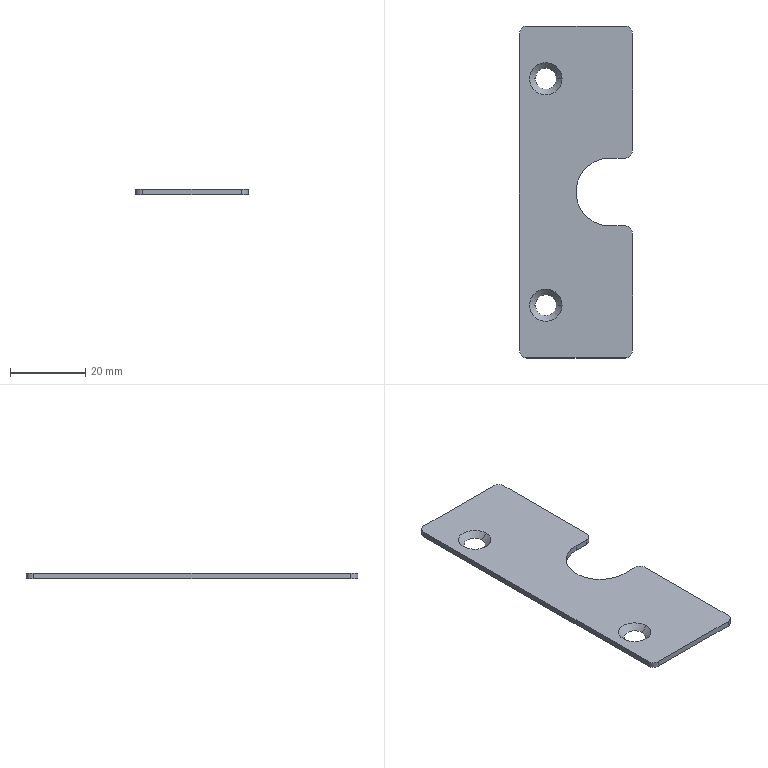Part | SolidWorks | features Chamfer 1, Fillet 1, FlatPattern 1, ICE 1, SMBaseFlange 1, SheetMetal 1 | 1 solid | 20 faces | box 30 x 88 x 1.5 mm | volume 3479 mm3 | plane 9 | cylinder 7 | cone 4 | commonest cylinder face diameters 4 x6 18 x1
STEP:
#1=CARTESIAN_POINT('',(-10.8,30.,-1.5));
#2=VERTEX_POINT('',#1);
#3=CARTESIAN_POINT('',(-5.2,30.,-1.5));
#4=VERTEX_POINT('',#3);
#5=CARTESIAN_POINT('',(-8.,30.,-1.5));
#6=DIRECTION('',(0.,0.,1.));
#7=DIRECTION('',(1.,0.,0.));
#8=AXIS2_PLACEMENT_3D('',#5,#6,#7);
#9=CIRCLE('',#8,2.8);
#10=EDGE_CURVE('',#2,#4,#9,.T.);
#11=ORIENTED_EDGE('',*,*,#10,.F.);
#12=CARTESIAN_POINT('',(-12.3,30.,0.));
#13=VERTEX_POINT('',#12);
#14=CARTESIAN_POINT('',(-10.8,30.,-1.5));
#15=DIRECTION('',(-0.7071,0.,0.7071));
#16=VECTOR('',#15,1000.);
#17=LINE('',#14,#16);
#18=EDGE_CURVE('',#2,#13,#17,.T.);
#19=ORIENTED_EDGE('',*,*,#18,.T.);
#20=CARTESIAN_POINT('',(-3.7,30.,0.));
#21=VERTEX_POINT('',#20);
#22=CARTESIAN_POINT('',(-8.,30.,0.));
#23=DIRECTION('',(0.,0.,-1.));
#24=DIRECTION('',(1.,0.,0.));
#25=AXIS2_PLACEMENT_3D('',#22,#23,#24);
#26=CIRCLE('',#25,4.3);
#27=EDGE_CURVE('',#21,#13,#26,.T.);
#28=ORIENTED_EDGE('',*,*,#27,.F.);
#29=CARTESIAN_POINT('',(-5.2,30.,-1.5));
#30=DIRECTION('',(0.7071,0.,0.7071));
#31=VECTOR('',#30,1000.);
#32=LINE('',#29,#31);
#33=EDGE_CURVE('',#4,#21,#32,.T.);
#34=ORIENTED_EDGE('',*,*,#33,.F.);
#35=EDGE_LOOP('',(#11,#19,#28,#34));
#36=FACE_OUTER_BOUND('',#35,.T.);
#37=CARTESIAN_POINT('',(-8.,30.,-1.5));
#38=DIRECTION('',(0.,0.,1.));
#39=DIRECTION('',(1.,0.,0.));
#40=AXIS2_PLACEMENT_3D('',#37,#38,#39);
#41=CONICAL_SURFACE('',#40,2.8,0.7854);
#42=ADVANCED_FACE('',(#36),#41,.F.);
#43=CARTESIAN_POINT('',(-10.8,-30.,-1.5));
#44=VERTEX_POINT('',#43);
#45=CARTESIAN_POINT('',(-5.2,-30.,-1.5));
#46=VERTEX_POINT('',#45);
#47=CARTESIAN_POINT('',(-8.,-30.,-1.5));
#48=DIRECTION('',(0.,0.,1.));
#49=DIRECTION('',(1.,0.,0.));
#50=AXIS2_PLACEMENT_3D('',#47,#48,#49);
#51=CIRCLE('',#50,2.8);
#52=EDGE_CURVE('',#44,#46,#51,.T.);
#53=ORIENTED_EDGE('',*,*,#52,.F.);
#54=CARTESIAN_POINT('',(-12.3,-30.,0.));
#55=VERTEX_POINT('',#54);
#56=CARTESIAN_POINT('',(-10.8,-30.,-1.5));
#57=DIRECTION('',(-0.7071,0.,0.7071));
#58=VECTOR('',#57,1000.);
#59=LINE('',#56,#58);
#60=EDGE_CURVE('',#44,#55,#59,.T.);
#61=ORIENTED_EDGE('',*,*,#60,.T.);
#62=CARTESIAN_POINT('',(-3.7,-30.,0.));
#63=VERTEX_POINT('',#62);
#64=CARTESIAN_POINT('',(-8.,-30.,0.));
#65=DIRECTION('',(0.,0.,-1.));
#66=DIRECTION('',(1.,0.,0.));
#67=AXIS2_PLACEMENT_3D('',#64,#65,#66);
#68=CIRCLE('',#67,4.3);
#69=EDGE_CURVE('',#63,#55,#68,.T.);
#70=ORIENTED_EDGE('',*,*,#69,.F.);
#71=CARTESIAN_POINT('',(-5.2,-30.,-1.5));
#72=DIRECTION('',(0.7071,0.,0.7071));
#73=VECTOR('',#72,1000.);
#74=LINE('',#71,#73);
#75=EDGE_CURVE('',#46,#63,#74,.T.);
#76=ORIENTED_EDGE('',*,*,#75,.F.);
#77=EDGE_LOOP('',(#53,#61,#70,#76));
#78=FACE_OUTER_BOUND('',#77,.T.);
#79=CARTESIAN_POINT('',(-8.,-30.,-1.5));
#80=DIRECTION('',(0.,0.,1.));
#81=DIRECTION('',(1.,0.,0.));
#82=AXIS2_PLACEMENT_3D('',#79,#80,#81);
#83=CONICAL_SURFACE('',#82,2.8,0.7854);
#84=ADVANCED_FACE('',(#78),#83,.F.);
#85=CARTESIAN_POINT('',(15.,11.,0.));
#86=VERTEX_POINT('',#85);
#87=CARTESIAN_POINT('',(15.,42.,0.));
#88=VERTEX_POINT('',#87);
#89=CARTESIAN_POINT('',(15.,44.,0.));
#90=DIRECTION('',(0.,1.,0.));
#91=VECTOR('',#90,1000.);
#92=LINE('',#89,#91);
#93=EDGE_CURVE('',#86,#88,#92,.T.);
#94=ORIENTED_EDGE('',*,*,#93,.F.);
#95=CARTESIAN_POINT('',(15.,11.,-1.5));
#96=VERTEX_POINT('',#95);
#97=CARTESIAN_POINT('',(15.,11.,-1.5));
#98=DIRECTION('',(0.,0.,-1.));
#99=VECTOR('',#98,1000.);
#100=LINE('',#97,#99);
#101=EDGE_CURVE('',#86,#96,#100,.T.);
#102=ORIENTED_EDGE('',*,*,#101,.T.);
#103=CARTESIAN_POINT('',(15.,42.,-1.5));
#104=VERTEX_POINT('',#103);
#105=CARTESIAN_POINT('',(15.,44.,-1.5));
#106=DIRECTION('',(0.,1.,0.));
#107=VECTOR('',#106,1000.);
#108=LINE('',#105,#107);
#109=EDGE_CURVE('',#96,#104,#108,.T.);
#110=ORIENTED_EDGE('',*,*,#109,.T.);
#111=CARTESIAN_POINT('',(15.,42.,-1.5));
#112=DIRECTION('',(0.,0.,1.));
#113=VECTOR('',#112,1000.);
#114=LINE('',#111,#113);
#115=EDGE_CURVE('',#104,#88,#114,.T.);
#116=ORIENTED_EDGE('',*,*,#115,.T.);
#117=EDGE_LOOP('',(#94,#102,#110,#116));
#118=FACE_OUTER_BOUND('',#117,.T.);
#119=CARTESIAN_POINT('',(15.,44.,-1.5));
#120=DIRECTION('',(1.,0.,0.));
#121=DIRECTION('',(0.,1.,0.));
#122=AXIS2_PLACEMENT_3D('',#119,#120,#121);
#123=PLANE('',#122);
#124=ADVANCED_FACE('',(#118),#123,.T.);
#125=CARTESIAN_POINT('',(15.,-42.,-1.5));
#126=VERTEX_POINT('',#125);
#127=CARTESIAN_POINT('',(15.,-11.,-1.5));
#128=VERTEX_POINT('',#127);
#129=CARTESIAN_POINT('',(15.,44.,-1.5));
#130=DIRECTION('',(0.,1.,0.));
#131=VECTOR('',#130,1000.);
#132=LINE('',#129,#131);
#133=EDGE_CURVE('',#126,#128,#132,.T.);
#134=ORIENTED_EDGE('',*,*,#133,.T.);
#135=CARTESIAN_POINT('',(15.,-11.,0.));
#136=VERTEX_POINT('',#135);
#137=CARTESIAN_POINT('',(15.,-11.,0.));
#138=DIRECTION('',(0.,0.,1.));
#139=VECTOR('',#138,1000.);
#140=LINE('',#137,#139);
#141=EDGE_CURVE('',#128,#136,#140,.T.);
#142=ORIENTED_EDGE('',*,*,#141,.T.);
#143=CARTESIAN_POINT('',(15.,-42.,0.));
#144=VERTEX_POINT('',#143);
#145=CARTESIAN_POINT('',(15.,44.,0.));
#146=DIRECTION('',(0.,1.,0.));
#147=VECTOR('',#146,1000.);
#148=LINE('',#145,#147);
#149=EDGE_CURVE('',#144,#136,#148,.T.);
#150=ORIENTED_EDGE('',*,*,#149,.F.);
#151=CARTESIAN_POINT('',(15.,-42.,-1.5));
#152=DIRECTION('',(0.,0.,-1.));
#153=VECTOR('',#152,1000.);
#154=LINE('',#151,#153);
#155=EDGE_CURVE('',#144,#126,#154,.T.);
#156=ORIENTED_EDGE('',*,*,#155,.T.);
#157=EDGE_LOOP('',(#134,#142,#150,#156));
#158=FACE_OUTER_BOUND('',#157,.T.);
#159=CARTESIAN_POINT('',(15.,44.,-1.5));
#160=DIRECTION('',(1.,0.,0.));
#161=DIRECTION('',(0.,1.,0.));
#162=AXIS2_PLACEMENT_3D('',#159,#160,#161);
#163=PLANE('',#162);
#164=ADVANCED_FACE('',(#158),#163,.T.);
#165=CARTESIAN_POINT('',(-13.,-44.,0.));
#166=VERTEX_POINT('',#165);
#167=CARTESIAN_POINT('',(13.,-44.,0.));
#168=VERTEX_POINT('',#167);
#169=CARTESIAN_POINT('',(-15.,-44.,0.));
#170=DIRECTION('',(1.,0.,0.));
#171=VECTOR('',#170,1000.);
#172=LINE('',#169,#171);
#173=EDGE_CURVE('',#166,#168,#172,.T.);
#174=ORIENTED_EDGE('',*,*,#173,.F.);
#175=CARTESIAN_POINT('',(-13.,-44.,-1.5));
#176=VERTEX_POINT('',#175);
#177=CARTESIAN_POINT('',(-13.,-44.,-1.5));
#178=DIRECTION('',(0.,0.,-1.));
#179=VECTOR('',#178,1000.);
#180=LINE('',#177,#179);
#181=EDGE_CURVE('',#166,#176,#180,.T.);
#182=ORIENTED_EDGE('',*,*,#181,.T.);
#183=CARTESIAN_POINT('',(13.,-44.,-1.5));
#184=VERTEX_POINT('',#183);
#185=CARTESIAN_POINT('',(-15.,-44.,-1.5));
#186=DIRECTION('',(1.,0.,0.));
#187=VECTOR('',#186,1000.);
#188=LINE('',#185,#187);
#189=EDGE_CURVE('',#176,#184,#188,.T.);
#190=ORIENTED_EDGE('',*,*,#189,.T.);
#191=CARTESIAN_POINT('',(13.,-44.,-1.5));
#192=DIRECTION('',(0.,0.,1.));
#193=VECTOR('',#192,1000.);
#194=LINE('',#191,#193);
#195=EDGE_CURVE('',#184,#168,#194,.T.);
#196=ORIENTED_EDGE('',*,*,#195,.T.);
#197=EDGE_LOOP('',(#174,#182,#190,#196));
#198=FACE_OUTER_BOUND('',#197,.T.);
#199=CARTESIAN_POINT('',(-15.,-44.,-1.5));
#200=DIRECTION('',(0.,-1.,0.));
#201=DIRECTION('',(0.,0.,-1.));
#202=AXIS2_PLACEMENT_3D('',#199,#200,#201);
#203=PLANE('',#202);
#204=ADVANCED_FACE('',(#198),#203,.T.);
#205=CARTESIAN_POINT('',(-15.,42.,-1.5));
#206=VERTEX_POINT('',#205);
#207=CARTESIAN_POINT('',(-15.,-42.,-1.5));
#208=VERTEX_POINT('',#207);
#209=CARTESIAN_POINT('',(-15.,44.,-1.5));
#210=DIRECTION('',(0.,-1.,0.));
#211=VECTOR('',#210,1000.);
#212=LINE('',#209,#211);
#213=EDGE_CURVE('',#206,#208,#212,.T.);
#214=ORIENTED_EDGE('',*,*,#213,.T.);
#215=CARTESIAN_POINT('',(-15.,-42.,0.));
#216=VERTEX_POINT('',#215);
#217=CARTESIAN_POINT('',(-15.,-42.,-1.5));
#218=DIRECTION('',(0.,0.,1.));
#219=VECTOR('',#218,1000.);
#220=LINE('',#217,#219);
#221=EDGE_CURVE('',#208,#216,#220,.T.);
#222=ORIENTED_EDGE('',*,*,#221,.T.);
#223=CARTESIAN_POINT('',(-15.,42.,0.));
#224=VERTEX_POINT('',#223);
#225=CARTESIAN_POINT('',(-15.,44.,0.));
#226=DIRECTION('',(0.,-1.,0.));
#227=VECTOR('',#226,1000.);
#228=LINE('',#225,#227);
#229=EDGE_CURVE('',#224,#216,#228,.T.);
#230=ORIENTED_EDGE('',*,*,#229,.F.);
#231=CARTESIAN_POINT('',(-15.,42.,-1.5));
#232=DIRECTION('',(0.,0.,-1.));
#233=VECTOR('',#232,1000.);
#234=LINE('',#231,#233);
#235=EDGE_CURVE('',#224,#206,#234,.T.);
#236=ORIENTED_EDGE('',*,*,#235,.T.);
#237=EDGE_LOOP('',(#214,#222,#230,#236));
#238=FACE_OUTER_BOUND('',#237,.T.);
#239=CARTESIAN_POINT('',(-15.,44.,-1.5));
#240=DIRECTION('',(-1.,0.,0.));
#241=DIRECTION('',(0.,-1.,0.));
#242=AXIS2_PLACEMENT_3D('',#239,#240,#241);
#243=PLANE('',#242);
#244=ADVANCED_FACE('',(#238),#243,.T.);
#245=CARTESIAN_POINT('',(13.,44.,-1.5));
#246=VERTEX_POINT('',#245);
#247=CARTESIAN_POINT('',(-13.,44.,-1.5));
#248=VERTEX_POINT('',#247);
#249=CARTESIAN_POINT('',(-15.,44.,-1.5));
#250=DIRECTION('',(-1.,0.,0.));
#251=VECTOR('',#250,1000.);
#252=LINE('',#249,#251);
#253=EDGE_CURVE('',#246,#248,#252,.T.);
#254=ORIENTED_EDGE('',*,*,#253,.T.);
#255=CARTESIAN_POINT('',(-13.,44.,0.));
#256=VERTEX_POINT('',#255);
#257=CARTESIAN_POINT('',(-13.,44.,-1.5));
#258=DIRECTION('',(0.,0.,1.));
#259=VECTOR('',#258,1000.);
#260=LINE('',#257,#259);
#261=EDGE_CURVE('',#248,#256,#260,.T.);
#262=ORIENTED_EDGE('',*,*,#261,.T.);
#263=CARTESIAN_POINT('',(13.,44.,0.));
#264=VERTEX_POINT('',#263);
#265=CARTESIAN_POINT('',(-15.,44.,0.));
#266=DIRECTION('',(-1.,0.,0.));
#267=VECTOR('',#266,1000.);
#268=LINE('',#265,#267);
#269=EDGE_CURVE('',#264,#256,#268,.T.);
#270=ORIENTED_EDGE('',*,*,#269,.F.);
#271=CARTESIAN_POINT('',(13.,44.,-1.5));
#272=DIRECTION('',(0.,0.,-1.));
#273=VECTOR('',#272,1000.);
#274=LINE('',#271,#273);
#275=EDGE_CURVE('',#264,#246,#274,.T.);
#276=ORIENTED_EDGE('',*,*,#275,.T.);
#277=EDGE_LOOP('',(#254,#262,#270,#276));
#278=FACE_OUTER_BOUND('',#277,.T.);
#279=CARTESIAN_POINT('',(-15.,44.,-1.5));
#280=DIRECTION('',(0.,1.,0.));
#281=DIRECTION('',(0.,0.,1.));
#282=AXIS2_PLACEMENT_3D('',#279,#280,#281);
#283=PLANE('',#282);
#284=ADVANCED_FACE('',(#278),#283,.T.);
#285=CARTESIAN_POINT('',(-8.,-30.,-1.5));
#286=DIRECTION('',(0.,0.,1.));
#287=DIRECTION('',(1.,0.,0.));
#288=AXIS2_PLACEMENT_3D('',#285,#286,#287);
#289=CIRCLE('',#288,2.8);
#290=EDGE_CURVE('',#46,#44,#289,.T.);
#291=ORIENTED_EDGE('',*,*,#290,.T.);
#292=ORIENTED_EDGE('',*,*,#52,.T.);
#293=EDGE_LOOP('',(#291,#292));
#294=FACE_BOUND('',#293,.T.);
#295=CARTESIAN_POINT('',(-8.,30.,-1.5));
#296=DIRECTION('',(0.,0.,1.));
#297=DIRECTION('',(1.,0.,0.));
#298=AXIS2_PLACEMENT_3D('',#295,#296,#297);
#299=CIRCLE('',#298,2.8);
#300=EDGE_CURVE('',#4,#2,#299,.T.);
#301=ORIENTED_EDGE('',*,*,#300,.T.);
#302=ORIENTED_EDGE('',*,*,#10,.T.);
#303=EDGE_LOOP('',(#301,#302));
#304=FACE_BOUND('',#303,.T.);
#305=CARTESIAN_POINT('',(9.,-9.,-1.5));
#306=VERTEX_POINT('',#305);
#307=CARTESIAN_POINT('',(13.,-9.,-1.5));
#308=VERTEX_POINT('',#307);
#309=CARTESIAN_POINT('',(0.,-9.,-1.5));
#310=DIRECTION('',(1.,0.,0.));
#311=VECTOR('',#310,1000.);
#312=LINE('',#309,#311);
#313=EDGE_CURVE('',#306,#308,#312,.T.);
#314=ORIENTED_EDGE('',*,*,#313,.T.);
#315=CARTESIAN_POINT('',(13.,-11.,-1.5));
#316=DIRECTION('',(0.,0.,-1.));
#317=DIRECTION('',(1.,0.,0.));
#318=AXIS2_PLACEMENT_3D('',#315,#316,#317);
#319=CIRCLE('',#318,2.);
#320=EDGE_CURVE('',#308,#128,#319,.T.);
#321=ORIENTED_EDGE('',*,*,#320,.T.);
#322=ORIENTED_EDGE('',*,*,#133,.F.);
#323=CARTESIAN_POINT('',(13.,-42.,-1.5));
#324=DIRECTION('',(0.,0.,-1.));
#325=DIRECTION('',(1.,0.,0.));
#326=AXIS2_PLACEMENT_3D('',#323,#324,#325);
#327=CIRCLE('',#326,2.);
#328=EDGE_CURVE('',#126,#184,#327,.T.);
#329=ORIENTED_EDGE('',*,*,#328,.T.);
#330=ORIENTED_EDGE('',*,*,#189,.F.);
#331=CARTESIAN_POINT('',(-13.,-42.,-1.5));
#332=DIRECTION('',(0.,0.,-1.));
#333=DIRECTION('',(1.,0.,0.));
#334=AXIS2_PLACEMENT_3D('',#331,#332,#333);
#335=CIRCLE('',#334,2.);
#336=EDGE_CURVE('',#176,#208,#335,.T.);
#337=ORIENTED_EDGE('',*,*,#336,.T.);
#338=ORIENTED_EDGE('',*,*,#213,.F.);
#339=CARTESIAN_POINT('',(-13.,42.,-1.5));
#340=DIRECTION('',(0.,0.,-1.));
#341=DIRECTION('',(1.,0.,0.));
#342=AXIS2_PLACEMENT_3D('',#339,#340,#341);
#343=CIRCLE('',#342,2.);
#344=EDGE_CURVE('',#206,#248,#343,.T.);
#345=ORIENTED_EDGE('',*,*,#344,.T.);
#346=ORIENTED_EDGE('',*,*,#253,.F.);
#347=CARTESIAN_POINT('',(13.,42.,-1.5));
#348=DIRECTION('',(0.,0.,-1.));
#349=DIRECTION('',(1.,0.,0.));
#350=AXIS2_PLACEMENT_3D('',#347,#348,#349);
#351=CIRCLE('',#350,2.);
#352=EDGE_CURVE('',#246,#104,#351,.T.);
#353=ORIENTED_EDGE('',*,*,#352,.T.);
#354=ORIENTED_EDGE('',*,*,#109,.F.);
#355=CARTESIAN_POINT('',(13.,9.,-1.5));
#356=VERTEX_POINT('',#355);
#357=CARTESIAN_POINT('',(13.,11.,-1.5));
#358=DIRECTION('',(0.,0.,-1.));
#359=DIRECTION('',(1.,0.,0.));
#360=AXIS2_PLACEMENT_3D('',#357,#358,#359);
#361=CIRCLE('',#360,2.);
#362=EDGE_CURVE('',#96,#356,#361,.T.);
#363=ORIENTED_EDGE('',*,*,#362,.T.);
#364=CARTESIAN_POINT('',(9.,9.,-1.5));
#365=VERTEX_POINT('',#364);
#366=CARTESIAN_POINT('',(0.,9.,-1.5));
#367=DIRECTION('',(-1.,0.,0.));
#368=VECTOR('',#367,1000.);
#369=LINE('',#366,#368);
#370=EDGE_CURVE('',#356,#365,#369,.T.);
#371=ORIENTED_EDGE('',*,*,#370,.T.);
#372=CARTESIAN_POINT('',(9.,0.,-1.5));
#373=DIRECTION('',(0.,0.,1.));
#374=DIRECTION('',(1.,0.,0.));
#375=AXIS2_PLACEMENT_3D('',#372,#373,#374);
#376=CIRCLE('',#375,9.);
#377=EDGE_CURVE('',#365,#306,#376,.T.);
#378=ORIENTED_EDGE('',*,*,#377,.T.);
#379=EDGE_LOOP('',(#314,#321,#322,#329,#330,#337,#338,#345,#346,#353,#354,#363,#371,#378));
#380=FACE_OUTER_BOUND('',#379,.T.);
#381=CARTESIAN_POINT('',(0.,0.,-1.5));
#382=DIRECTION('',(0.,0.,1.));
#383=DIRECTION('',(1.,0.,0.));
#384=AXIS2_PLACEMENT_3D('',#381,#382,#383);
#385=PLANE('',#384);
#386=ADVANCED_FACE('',(#294,#304,#380),#385,.F.);
#387=ORIENTED_EDGE('',*,*,#69,.T.);
#388=CARTESIAN_POINT('',(-8.,-30.,0.));
#389=DIRECTION('',(0.,0.,-1.));
#390=DIRECTION('',(1.,0.,0.));
#391=AXIS2_PLACEMENT_3D('',#388,#389,#390);
#392=CIRCLE('',#391,4.3);
#393=EDGE_CURVE('',#55,#63,#392,.T.);
#394=ORIENTED_EDGE('',*,*,#393,.T.);
#395=EDGE_LOOP('',(#387,#394));
#396=FACE_BOUND('',#395,.T.);
#397=ORIENTED_EDGE('',*,*,#27,.T.);
#398=CARTESIAN_POINT('',(-8.,30.,0.));
#399=DIRECTION('',(0.,0.,-1.));
#400=DIRECTION('',(1.,0.,0.));
#401=AXIS2_PLACEMENT_3D('',#398,#399,#400);
#402=CIRCLE('',#401,4.3);
#403=EDGE_CURVE('',#13,#21,#402,.T.);
#404=ORIENTED_EDGE('',*,*,#403,.T.);
#405=EDGE_LOOP('',(#397,#404));
#406=FACE_BOUND('',#405,.T.);
#407=ORIENTED_EDGE('',*,*,#149,.T.);
#408=CARTESIAN_POINT('',(13.,-9.,0.));
#409=VERTEX_POINT('',#408);
#410=CARTESIAN_POINT('',(13.,-11.,0.));
#411=DIRECTION('',(0.,0.,1.));
#412=DIRECTION('',(1.,0.,0.));
#413=AXIS2_PLACEMENT_3D('',#410,#411,#412);
#414=CIRCLE('',#413,2.);
#415=EDGE_CURVE('',#136,#409,#414,.T.);
#416=ORIENTED_EDGE('',*,*,#415,.T.);
#417=CARTESIAN_POINT('',(9.,-9.,0.));
#418=VERTEX_POINT('',#417);
#419=CARTESIAN_POINT('',(9.,-9.,0.));
#420=DIRECTION('',(1.,0.,0.));
#421=VECTOR('',#420,1000.);
#422=LINE('',#419,#421);
#423=EDGE_CURVE('',#418,#409,#422,.T.);
#424=ORIENTED_EDGE('',*,*,#423,.F.);
#425=CARTESIAN_POINT('',(9.,9.,0.));
#426=VERTEX_POINT('',#425);
#427=CARTESIAN_POINT('',(9.,0.,0.));
#428=DIRECTION('',(0.,0.,1.));
#429=DIRECTION('',(1.,0.,0.));
#430=AXIS2_PLACEMENT_3D('',#427,#428,#429);
#431=CIRCLE('',#430,9.);
#432=EDGE_CURVE('',#426,#418,#431,.T.);
#433=ORIENTED_EDGE('',*,*,#432,.F.);
#434=CARTESIAN_POINT('',(13.,9.,0.));
#435=VERTEX_POINT('',#434);
#436=CARTESIAN_POINT('',(9.,9.,0.));
#437=DIRECTION('',(-1.,0.,0.));
#438=VECTOR('',#437,1000.);
#439=LINE('',#436,#438);
#440=EDGE_CURVE('',#435,#426,#439,.T.);
#441=ORIENTED_EDGE('',*,*,#440,.F.);
#442=CARTESIAN_POINT('',(13.,11.,0.));
#443=DIRECTION('',(0.,0.,1.));
#444=DIRECTION('',(1.,0.,0.));
#445=AXIS2_PLACEMENT_3D('',#442,#443,#444);
#446=CIRCLE('',#445,2.);
#447=EDGE_CURVE('',#435,#86,#446,.T.);
#448=ORIENTED_EDGE('',*,*,#447,.T.);
#449=ORIENTED_EDGE('',*,*,#93,.T.);
#450=CARTESIAN_POINT('',(13.,42.,0.));
#451=DIRECTION('',(0.,0.,1.));
#452=DIRECTION('',(1.,0.,0.));
#453=AXIS2_PLACEMENT_3D('',#450,#451,#452);
#454=CIRCLE('',#453,2.);
#455=EDGE_CURVE('',#88,#264,#454,.T.);
#456=ORIENTED_EDGE('',*,*,#455,.T.);
#457=ORIENTED_EDGE('',*,*,#269,.T.);
#458=CARTESIAN_POINT('',(-13.,42.,0.));
#459=DIRECTION('',(0.,0.,1.));
#460=DIRECTION('',(1.,0.,0.));
#461=AXIS2_PLACEMENT_3D('',#458,#459,#460);
#462=CIRCLE('',#461,2.);
#463=EDGE_CURVE('',#256,#224,#462,.T.);
#464=ORIENTED_EDGE('',*,*,#463,.T.);
#465=ORIENTED_EDGE('',*,*,#229,.T.);
#466=CARTESIAN_POINT('',(-13.,-42.,0.));
#467=DIRECTION('',(0.,0.,1.));
#468=DIRECTION('',(1.,0.,0.));
#469=AXIS2_PLACEMENT_3D('',#466,#467,#468);
#470=CIRCLE('',#469,2.);
#471=EDGE_CURVE('',#216,#166,#470,.T.);
#472=ORIENTED_EDGE('',*,*,#471,.T.);
#473=ORIENTED_EDGE('',*,*,#173,.T.);
#474=CARTESIAN_POINT('',(13.,-42.,0.));
#475=DIRECTION('',(0.,0.,1.));
#476=DIRECTION('',(1.,0.,0.));
#477=AXIS2_PLACEMENT_3D('',#474,#475,#476);
#478=CIRCLE('',#477,2.);
#479=EDGE_CURVE('',#168,#144,#478,.T.);
#480=ORIENTED_EDGE('',*,*,#479,.T.);
#481=EDGE_LOOP('',(#407,#416,#424,#433,#441,#448,#449,#456,#457,#464,#465,#472,#473,#480));
#482=FACE_OUTER_BOUND('',#481,.T.);
#483=CARTESIAN_POINT('',(0.,0.,0.));
#484=DIRECTION('',(0.,0.,1.));
#485=DIRECTION('',(1.,0.,0.));
#486=AXIS2_PLACEMENT_3D('',#483,#484,#485);
#487=PLANE('',#486);
#488=ADVANCED_FACE('',(#396,#406,#482),#487,.T.);
#489=CARTESIAN_POINT('',(9.,9.,-10.));
#490=DIRECTION('',(0.,0.,1.));
#491=VECTOR('',#490,1000.);
#492=LINE('',#489,#491);
#493=EDGE_CURVE('',#365,#426,#492,.T.);
#494=ORIENTED_EDGE('',*,*,#493,.T.);
#495=ORIENTED_EDGE('',*,*,#432,.T.);
#496=CARTESIAN_POINT('',(9.,-9.,-10.));
#497=DIRECTION('',(0.,0.,1.));
#498=VECTOR('',#497,1000.);
#499=LINE('',#496,#498);
#500=EDGE_CURVE('',#306,#418,#499,.T.);
#501=ORIENTED_EDGE('',*,*,#500,.F.);
#502=ORIENTED_EDGE('',*,*,#377,.F.);
#503=EDGE_LOOP('',(#494,#495,#501,#502));
#504=FACE_OUTER_BOUND('',#503,.T.);
#505=CARTESIAN_POINT('',(9.,0.,-10.));
#506=DIRECTION('',(0.,0.,1.));
#507=DIRECTION('',(1.,0.,0.));
#508=AXIS2_PLACEMENT_3D('',#505,#506,#507);
#509=CYLINDRICAL_SURFACE('',#508,9.);
#510=ADVANCED_FACE('',(#504),#509,.F.);
#511=ORIENTED_EDGE('',*,*,#370,.F.);
#512=CARTESIAN_POINT('',(13.,9.,0.));
#513=DIRECTION('',(0.,0.,1.));
#514=VECTOR('',#513,1000.);
#515=LINE('',#512,#514);
#516=EDGE_CURVE('',#356,#435,#515,.T.);
#517=ORIENTED_EDGE('',*,*,#516,.T.);
#518=ORIENTED_EDGE('',*,*,#440,.T.);
#519=ORIENTED_EDGE('',*,*,#493,.F.);
#520=EDGE_LOOP('',(#511,#517,#518,#519));
#521=FACE_OUTER_BOUND('',#520,.T.);
#522=CARTESIAN_POINT('',(9.,9.,-10.));
#523=DIRECTION('',(0.,1.,0.));
#524=DIRECTION('',(-1.,0.,0.));
#525=AXIS2_PLACEMENT_3D('',#522,#523,#524);
#526=PLANE('',#525);
#527=ADVANCED_FACE('',(#521),#526,.F.);
#528=ORIENTED_EDGE('',*,*,#423,.T.);
#529=CARTESIAN_POINT('',(13.,-9.,-1.5));
#530=DIRECTION('',(0.,0.,-1.));
#531=VECTOR('',#530,1000.);
#532=LINE('',#529,#531);
#533=EDGE_CURVE('',#409,#308,#532,.T.);
#534=ORIENTED_EDGE('',*,*,#533,.T.);
#535=ORIENTED_EDGE('',*,*,#313,.F.);
#536=ORIENTED_EDGE('',*,*,#500,.T.);
#537=EDGE_LOOP('',(#528,#534,#535,#536));
#538=FACE_OUTER_BOUND('',#537,.T.);
#539=CARTESIAN_POINT('',(9.,-9.,-10.));
#540=DIRECTION('',(0.,-1.,0.));
#541=DIRECTION('',(1.,0.,0.));
#542=AXIS2_PLACEMENT_3D('',#539,#540,#541);
#543=PLANE('',#542);
#544=ADVANCED_FACE('',(#538),#543,.F.);
#545=ORIENTED_EDGE('',*,*,#320,.F.);
#546=ORIENTED_EDGE('',*,*,#533,.F.);
#547=ORIENTED_EDGE('',*,*,#415,.F.);
#548=ORIENTED_EDGE('',*,*,#141,.F.);
#549=EDGE_LOOP('',(#545,#546,#547,#548));
#550=FACE_OUTER_BOUND('',#549,.T.);
#551=CARTESIAN_POINT('',(13.,-11.,-1.5));
#552=DIRECTION('',(0.,0.,-1.));
#553=DIRECTION('',(-1.,0.,0.));
#554=AXIS2_PLACEMENT_3D('',#551,#552,#553);
#555=CYLINDRICAL_SURFACE('',#554,2.);
#556=ADVANCED_FACE('',(#550),#555,.T.);
#557=ORIENTED_EDGE('',*,*,#362,.F.);
#558=ORIENTED_EDGE('',*,*,#101,.F.);
#559=ORIENTED_EDGE('',*,*,#447,.F.);
#560=ORIENTED_EDGE('',*,*,#516,.F.);
#561=EDGE_LOOP('',(#557,#558,#559,#560));
#562=FACE_OUTER_BOUND('',#561,.T.);
#563=CARTESIAN_POINT('',(13.,11.,-10.));
#564=DIRECTION('',(0.,0.,-1.));
#565=DIRECTION('',(-1.,0.,0.));
#566=AXIS2_PLACEMENT_3D('',#563,#564,#565);
#567=CYLINDRICAL_SURFACE('',#566,2.);
#568=ADVANCED_FACE('',(#562),#567,.T.);
#569=ORIENTED_EDGE('',*,*,#336,.F.);
#570=ORIENTED_EDGE('',*,*,#181,.F.);
#571=ORIENTED_EDGE('',*,*,#471,.F.);
#572=ORIENTED_EDGE('',*,*,#221,.F.);
#573=EDGE_LOOP('',(#569,#570,#571,#572));
#574=FACE_OUTER_BOUND('',#573,.T.);
#575=CARTESIAN_POINT('',(-13.,-42.,-1.5));
#576=DIRECTION('',(0.,0.,1.));
#577=DIRECTION('',(1.,0.,0.));
#578=AXIS2_PLACEMENT_3D('',#575,#576,#577);
#579=CYLINDRICAL_SURFACE('',#578,2.);
#580=ADVANCED_FACE('',(#574),#579,.T.);
#581=ORIENTED_EDGE('',*,*,#328,.F.);
#582=ORIENTED_EDGE('',*,*,#155,.F.);
#583=ORIENTED_EDGE('',*,*,#479,.F.);
#584=ORIENTED_EDGE('',*,*,#195,.F.);
#585=EDGE_LOOP('',(#581,#582,#583,#584));
#586=FACE_OUTER_BOUND('',#585,.T.);
#587=CARTESIAN_POINT('',(13.,-42.,-1.5));
#588=DIRECTION('',(0.,0.,1.));
#589=DIRECTION('',(1.,0.,0.));
#590=AXIS2_PLACEMENT_3D('',#587,#588,#589);
#591=CYLINDRICAL_SURFACE('',#590,2.);
#592=ADVANCED_FACE('',(#586),#591,.T.);
#593=ORIENTED_EDGE('',*,*,#344,.F.);
#594=ORIENTED_EDGE('',*,*,#235,.F.);
#595=ORIENTED_EDGE('',*,*,#463,.F.);
#596=ORIENTED_EDGE('',*,*,#261,.F.);
#597=EDGE_LOOP('',(#593,#594,#595,#596));
#598=FACE_OUTER_BOUND('',#597,.T.);
#599=CARTESIAN_POINT('',(-13.,42.,-1.5));
#600=DIRECTION('',(0.,0.,1.));
#601=DIRECTION('',(1.,0.,0.));
#602=AXIS2_PLACEMENT_3D('',#599,#600,#601);
#603=CYLINDRICAL_SURFACE('',#602,2.);
#604=ADVANCED_FACE('',(#598),#603,.T.);
#605=ORIENTED_EDGE('',*,*,#352,.F.);
#606=ORIENTED_EDGE('',*,*,#275,.F.);
#607=ORIENTED_EDGE('',*,*,#455,.F.);
#608=ORIENTED_EDGE('',*,*,#115,.F.);
#609=EDGE_LOOP('',(#605,#606,#607,#608));
#610=FACE_OUTER_BOUND('',#609,.T.);
#611=CARTESIAN_POINT('',(13.,42.,-1.5));
#612=DIRECTION('',(0.,0.,1.));
#613=DIRECTION('',(1.,0.,0.));
#614=AXIS2_PLACEMENT_3D('',#611,#612,#613);
#615=CYLINDRICAL_SURFACE('',#614,2.);
#616=ADVANCED_FACE('',(#610),#615,.T.);
#617=ORIENTED_EDGE('',*,*,#60,.F.);
#618=ORIENTED_EDGE('',*,*,#290,.F.);
#619=ORIENTED_EDGE('',*,*,#75,.T.);
#620=ORIENTED_EDGE('',*,*,#393,.F.);
#621=EDGE_LOOP('',(#617,#618,#619,#620));
#622=FACE_OUTER_BOUND('',#621,.T.);
#623=CARTESIAN_POINT('',(-8.,-30.,-1.5));
#624=DIRECTION('',(0.,0.,1.));
#625=DIRECTION('',(1.,0.,0.));
#626=AXIS2_PLACEMENT_3D('',#623,#624,#625);
#627=CONICAL_SURFACE('',#626,2.8,0.7854);
#628=ADVANCED_FACE('',(#622),#627,.F.);
#629=ORIENTED_EDGE('',*,*,#18,.F.);
#630=ORIENTED_EDGE('',*,*,#300,.F.);
#631=ORIENTED_EDGE('',*,*,#33,.T.);
#632=ORIENTED_EDGE('',*,*,#403,.F.);
#633=EDGE_LOOP('',(#629,#630,#631,#632));
#634=FACE_OUTER_BOUND('',#633,.T.);
#635=CARTESIAN_POINT('',(-8.,30.,-1.5));
#636=DIRECTION('',(0.,0.,1.));
#637=DIRECTION('',(1.,0.,0.));
#638=AXIS2_PLACEMENT_3D('',#635,#636,#637);
#639=CONICAL_SURFACE('',#638,2.8,0.7854);
#640=ADVANCED_FACE('',(#634),#639,.F.);
#641=CLOSED_SHELL('',(#42,#84,#124,#164,#204,#244,#284,#386,#488,#510,#527,#544,#556,#568,#580,#592,#604,#616,#628,#640));
#642=MANIFOLD_SOLID_BREP('',#641);
#643=CARTESIAN_POINT('',(0.,0.,0.));
#644=DIRECTION('',(0.,0.,1.));
#645=DIRECTION('',(1.,0.,0.));
#646=AXIS2_PLACEMENT_3D('',#643,#644,#645);
#647=(LENGTH_UNIT()NAMED_UNIT(*)SI_UNIT(.MILLI.,.METRE.));
#648=UNCERTAINTY_MEASURE_WITH_UNIT(LENGTH_MEASURE(0.00001),#647,'','');
#649=(NAMED_UNIT(*)PLANE_ANGLE_UNIT()SI_UNIT($,.RADIAN.));
#650=(NAMED_UNIT(*)SI_UNIT($,.STERADIAN.)SOLID_ANGLE_UNIT());
#651=(GEOMETRIC_REPRESENTATION_CONTEXT(3)GLOBAL_UNCERTAINTY_ASSIGNED_CONTEXT((#648))GLOBAL_UNIT_ASSIGNED_CONTEXT((#647,#649,#650))REPRESENTATION_CONTEXT('',''));
#652=ADVANCED_BREP_SHAPE_REPRESENTATION('',(#642,#646),#651);